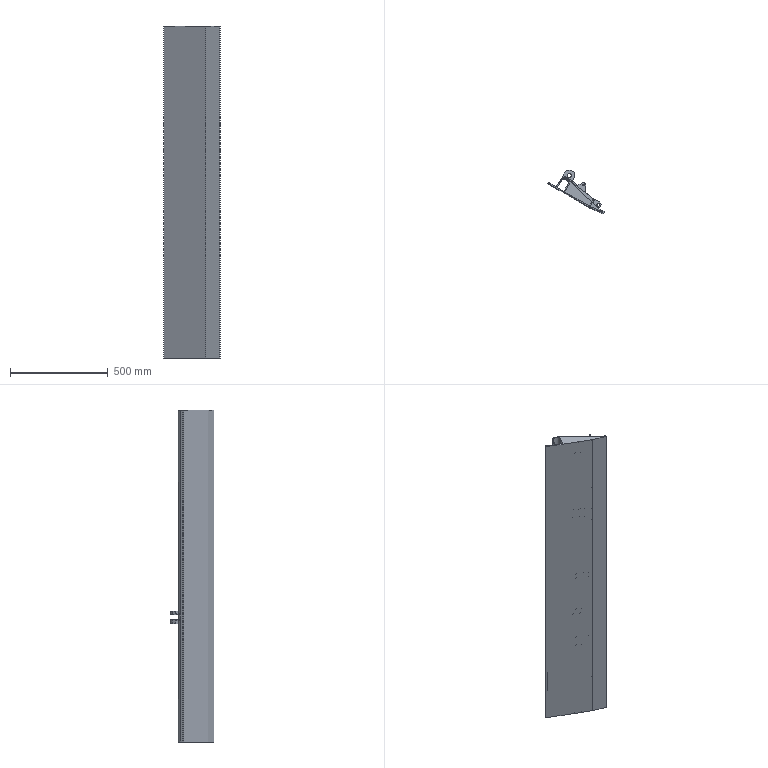Part | SolidWorks | features ICE 26, Extrusion 1 | 1 solid | 164 faces | box 289.155 x 223.548 x 1700 mm | volume 5050781 mm3 | plane 130 | cylinder 34 | commonest cylinder face diameters 10 x8 15 x8 50 x5 20 x4 55 x3 3 x2